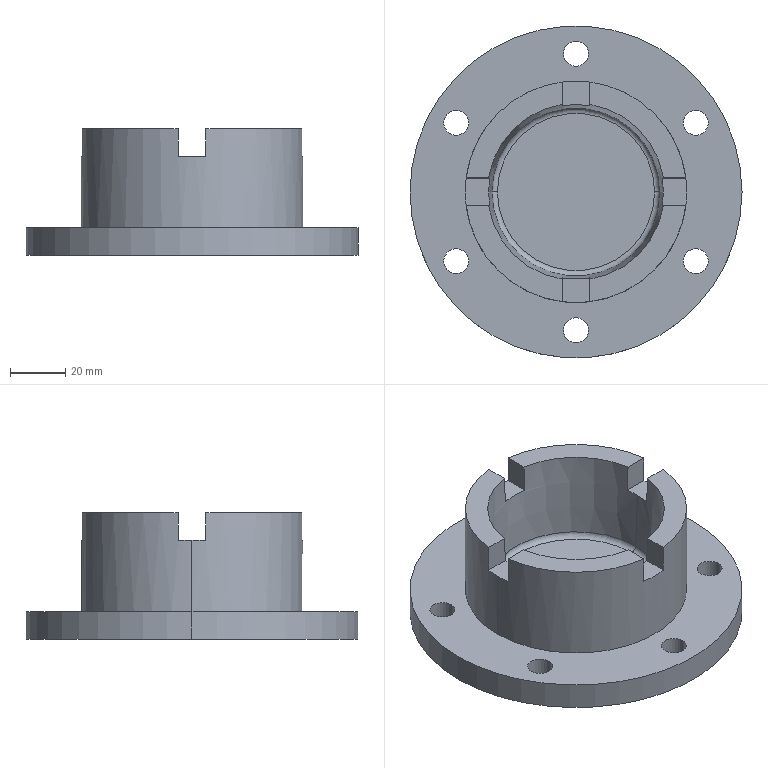Part | SolidWorks | features ICE 5, CirPattern 2, Fillet 1, Revolution 1 | 1 solid | 948 faces | box 120 x 120 x 45.75 mm | volume 173021 mm3 | plane 691 | spline 235 | cylinder 16 | torus 4 | cone 2 | commonest cylinder face diameters 9 x12 80 x2 120 x2